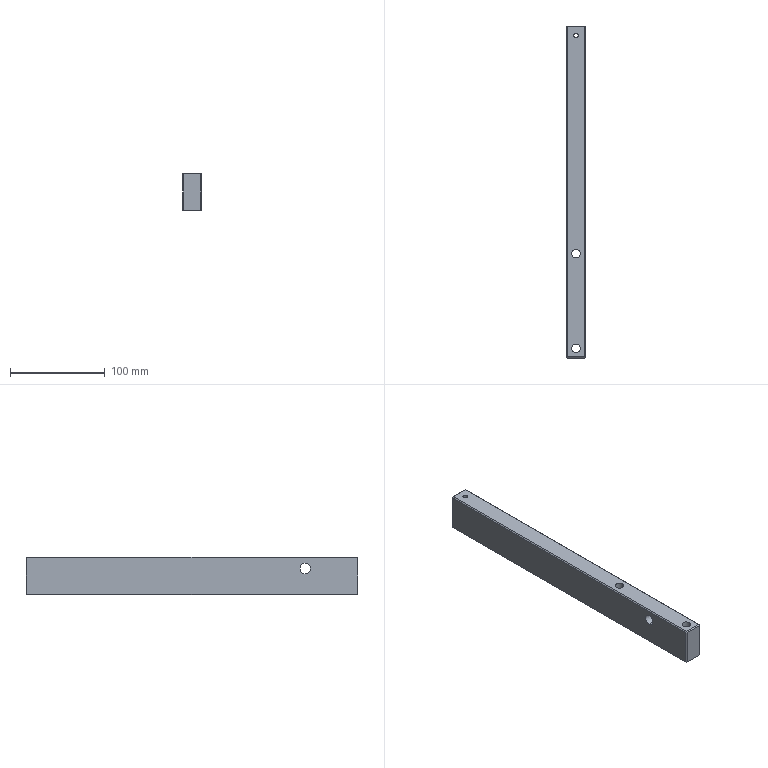Part | SolidWorks | features HoleWzd 3, Chamfer 1, Extrusion 1, ICE 1 | 1 solid | 48 faces | box 20 x 350 x 40 mm | volume 265293 mm3 | plane 30 | cylinder 18 | commonest cylinder face diameters 5 x4 9 x4 15 x4 11 x2 12.8 x2 18 x2
STEP:
#1=CARTESIAN_POINT('',(-1.,55.662,17.));
#2=VERTEX_POINT('',#1);
#3=CARTESIAN_POINT('',(-1.,55.662,-1.));
#4=VERTEX_POINT('',#3);
#5=CARTESIAN_POINT('',(-1.,55.662,8.));
#6=DIRECTION('',(1.,0.,0.));
#7=DIRECTION('',(0.,0.,-1.));
#8=AXIS2_PLACEMENT_3D('',#5,#6,#7);
#9=CIRCLE('',#8,9.);
#10=EDGE_CURVE('',#2,#4,#9,.T.);
#11=ORIENTED_EDGE('',*,*,#10,.F.);
#12=CARTESIAN_POINT('',(10.,55.662,17.));
#13=VERTEX_POINT('',#12);
#14=CARTESIAN_POINT('',(10.,55.662,17.));
#15=DIRECTION('',(1.,0.,0.));
#16=VECTOR('',#15,1000.);
#17=LINE('',#14,#16);
#18=EDGE_CURVE('',#2,#13,#17,.T.);
#19=ORIENTED_EDGE('',*,*,#18,.T.);
#20=CARTESIAN_POINT('',(10.,55.662,-1.));
#21=VERTEX_POINT('',#20);
#22=CARTESIAN_POINT('',(10.,55.662,8.));
#23=DIRECTION('',(1.,0.,0.));
#24=DIRECTION('',(0.,0.,-1.));
#25=AXIS2_PLACEMENT_3D('',#22,#23,#24);
#26=CIRCLE('',#25,9.);
#27=EDGE_CURVE('',#13,#21,#26,.T.);
#28=ORIENTED_EDGE('',*,*,#27,.T.);
#29=CARTESIAN_POINT('',(10.,55.662,-1.));
#30=DIRECTION('',(1.,0.,0.));
#31=VECTOR('',#30,1000.);
#32=LINE('',#29,#31);
#33=EDGE_CURVE('',#4,#21,#32,.T.);
#34=ORIENTED_EDGE('',*,*,#33,.F.);
#35=EDGE_LOOP('',(#11,#19,#28,#34));
#36=FACE_OUTER_BOUND('',#35,.T.);
#37=CARTESIAN_POINT('',(10.,55.662,8.));
#38=DIRECTION('',(1.,0.,0.));
#39=DIRECTION('',(0.,0.,-1.));
#40=AXIS2_PLACEMENT_3D('',#37,#38,#39);
#41=CYLINDRICAL_SURFACE('',#40,9.);
#42=ADVANCED_FACE('',(#36),#41,.F.);
#43=CARTESIAN_POINT('',(-10.,55.662,13.5));
#44=VERTEX_POINT('',#43);
#45=CARTESIAN_POINT('',(-10.,55.662,2.5));
#46=VERTEX_POINT('',#45);
#47=CARTESIAN_POINT('',(-10.,55.662,8.));
#48=DIRECTION('',(1.,0.,0.));
#49=DIRECTION('',(0.,0.,-1.));
#50=AXIS2_PLACEMENT_3D('',#47,#48,#49);
#51=CIRCLE('',#50,5.5);
#52=EDGE_CURVE('',#44,#46,#51,.T.);
#53=ORIENTED_EDGE('',*,*,#52,.F.);
#54=CARTESIAN_POINT('',(-1.,55.662,13.5));
#55=VERTEX_POINT('',#54);
#56=CARTESIAN_POINT('',(10.,55.662,13.5));
#57=DIRECTION('',(1.,0.,0.));
#58=VECTOR('',#57,1000.);
#59=LINE('',#56,#58);
#60=EDGE_CURVE('',#44,#55,#59,.T.);
#61=ORIENTED_EDGE('',*,*,#60,.T.);
#62=CARTESIAN_POINT('',(-1.,55.662,2.5));
#63=VERTEX_POINT('',#62);
#64=CARTESIAN_POINT('',(-1.,55.662,8.));
#65=DIRECTION('',(1.,0.,0.));
#66=DIRECTION('',(0.,0.,-1.));
#67=AXIS2_PLACEMENT_3D('',#64,#65,#66);
#68=CIRCLE('',#67,5.5);
#69=EDGE_CURVE('',#55,#63,#68,.T.);
#70=ORIENTED_EDGE('',*,*,#69,.T.);
#71=CARTESIAN_POINT('',(10.,55.662,2.5));
#72=DIRECTION('',(1.,0.,0.));
#73=VECTOR('',#72,1000.);
#74=LINE('',#71,#73);
#75=EDGE_CURVE('',#46,#63,#74,.T.);
#76=ORIENTED_EDGE('',*,*,#75,.F.);
#77=EDGE_LOOP('',(#53,#61,#70,#76));
#78=FACE_OUTER_BOUND('',#77,.T.);
#79=CARTESIAN_POINT('',(10.,55.662,8.));
#80=DIRECTION('',(1.,0.,0.));
#81=DIRECTION('',(0.,0.,-1.));
#82=AXIS2_PLACEMENT_3D('',#79,#80,#81);
#83=CYLINDRICAL_SURFACE('',#82,5.5);
#84=ADVANCED_FACE('',(#78),#83,.F.);
#85=CARTESIAN_POINT('',(7.5,10.,-11.));
#86=VERTEX_POINT('',#85);
#87=CARTESIAN_POINT('',(-7.5,10.,-11.));
#88=VERTEX_POINT('',#87);
#89=CARTESIAN_POINT('',(0.,10.,-11.));
#90=DIRECTION('',(0.,0.,-1.));
#91=DIRECTION('',(-1.,0.,0.));
#92=AXIS2_PLACEMENT_3D('',#89,#90,#91);
#93=CIRCLE('',#92,7.5);
#94=EDGE_CURVE('',#86,#88,#93,.T.);
#95=ORIENTED_EDGE('',*,*,#94,.F.);
#96=CARTESIAN_POINT('',(7.5,10.,-20.));
#97=VERTEX_POINT('',#96);
#98=CARTESIAN_POINT('',(7.5,10.,-20.));
#99=DIRECTION('',(0.,0.,-1.));
#100=VECTOR('',#99,1000.);
#101=LINE('',#98,#100);
#102=EDGE_CURVE('',#86,#97,#101,.T.);
#103=ORIENTED_EDGE('',*,*,#102,.T.);
#104=CARTESIAN_POINT('',(-7.5,10.,-20.));
#105=VERTEX_POINT('',#104);
#106=CARTESIAN_POINT('',(0.,10.,-20.));
#107=DIRECTION('',(0.,0.,-1.));
#108=DIRECTION('',(-1.,0.,0.));
#109=AXIS2_PLACEMENT_3D('',#106,#107,#108);
#110=CIRCLE('',#109,7.5);
#111=EDGE_CURVE('',#97,#105,#110,.T.);
#112=ORIENTED_EDGE('',*,*,#111,.T.);
#113=CARTESIAN_POINT('',(-7.5,10.,-20.));
#114=DIRECTION('',(0.,0.,-1.));
#115=VECTOR('',#114,1000.);
#116=LINE('',#113,#115);
#117=EDGE_CURVE('',#88,#105,#116,.T.);
#118=ORIENTED_EDGE('',*,*,#117,.F.);
#119=EDGE_LOOP('',(#95,#103,#112,#118));
#120=FACE_OUTER_BOUND('',#119,.T.);
#121=CARTESIAN_POINT('',(0.,10.,-20.));
#122=DIRECTION('',(0.,0.,-1.));
#123=DIRECTION('',(-1.,0.,0.));
#124=AXIS2_PLACEMENT_3D('',#121,#122,#123);
#125=CYLINDRICAL_SURFACE('',#124,7.5);
#126=ADVANCED_FACE('',(#120),#125,.F.);
#127=CARTESIAN_POINT('',(4.5,10.,20.));
#128=VERTEX_POINT('',#127);
#129=CARTESIAN_POINT('',(-4.5,10.,20.));
#130=VERTEX_POINT('',#129);
#131=CARTESIAN_POINT('',(0.,10.,20.));
#132=DIRECTION('',(0.,0.,-1.));
#133=DIRECTION('',(-1.,0.,0.));
#134=AXIS2_PLACEMENT_3D('',#131,#132,#133);
#135=CIRCLE('',#134,4.5);
#136=EDGE_CURVE('',#128,#130,#135,.T.);
#137=ORIENTED_EDGE('',*,*,#136,.F.);
#138=CARTESIAN_POINT('',(4.5,10.,-11.));
#139=VERTEX_POINT('',#138);
#140=CARTESIAN_POINT('',(4.5,10.,-20.));
#141=DIRECTION('',(0.,0.,-1.));
#142=VECTOR('',#141,1000.);
#143=LINE('',#140,#142);
#144=EDGE_CURVE('',#128,#139,#143,.T.);
#145=ORIENTED_EDGE('',*,*,#144,.T.);
#146=CARTESIAN_POINT('',(-4.5,10.,-11.));
#147=VERTEX_POINT('',#146);
#148=CARTESIAN_POINT('',(0.,10.,-11.));
#149=DIRECTION('',(0.,0.,-1.));
#150=DIRECTION('',(-1.,0.,0.));
#151=AXIS2_PLACEMENT_3D('',#148,#149,#150);
#152=CIRCLE('',#151,4.5);
#153=EDGE_CURVE('',#139,#147,#152,.T.);
#154=ORIENTED_EDGE('',*,*,#153,.T.);
#155=CARTESIAN_POINT('',(-4.5,10.,-20.));
#156=DIRECTION('',(0.,0.,-1.));
#157=VECTOR('',#156,1000.);
#158=LINE('',#155,#157);
#159=EDGE_CURVE('',#130,#147,#158,.T.);
#160=ORIENTED_EDGE('',*,*,#159,.F.);
#161=EDGE_LOOP('',(#137,#145,#154,#160));
#162=FACE_OUTER_BOUND('',#161,.T.);
#163=CARTESIAN_POINT('',(0.,10.,-20.));
#164=DIRECTION('',(0.,0.,-1.));
#165=DIRECTION('',(-1.,0.,0.));
#166=AXIS2_PLACEMENT_3D('',#163,#164,#165);
#167=CYLINDRICAL_SURFACE('',#166,4.5);
#168=ADVANCED_FACE('',(#162),#167,.F.);
#169=CARTESIAN_POINT('',(7.5,110.,-11.));
#170=VERTEX_POINT('',#169);
#171=CARTESIAN_POINT('',(-7.5,110.,-11.));
#172=VERTEX_POINT('',#171);
#173=CARTESIAN_POINT('',(0.,110.,-11.));
#174=DIRECTION('',(0.,0.,-1.));
#175=DIRECTION('',(-1.,0.,0.));
#176=AXIS2_PLACEMENT_3D('',#173,#174,#175);
#177=CIRCLE('',#176,7.5);
#178=EDGE_CURVE('',#170,#172,#177,.T.);
#179=ORIENTED_EDGE('',*,*,#178,.F.);
#180=CARTESIAN_POINT('',(7.5,110.,-20.));
#181=VERTEX_POINT('',#180);
#182=CARTESIAN_POINT('',(7.5,110.,-20.));
#183=DIRECTION('',(0.,0.,-1.));
#184=VECTOR('',#183,1000.);
#185=LINE('',#182,#184);
#186=EDGE_CURVE('',#170,#181,#185,.T.);
#187=ORIENTED_EDGE('',*,*,#186,.T.);
#188=CARTESIAN_POINT('',(-7.5,110.,-20.));
#189=VERTEX_POINT('',#188);
#190=CARTESIAN_POINT('',(0.,110.,-20.));
#191=DIRECTION('',(0.,0.,-1.));
#192=DIRECTION('',(-1.,0.,0.));
#193=AXIS2_PLACEMENT_3D('',#190,#191,#192);
#194=CIRCLE('',#193,7.5);
#195=EDGE_CURVE('',#181,#189,#194,.T.);
#196=ORIENTED_EDGE('',*,*,#195,.T.);
#197=CARTESIAN_POINT('',(-7.5,110.,-20.));
#198=DIRECTION('',(0.,0.,-1.));
#199=VECTOR('',#198,1000.);
#200=LINE('',#197,#199);
#201=EDGE_CURVE('',#172,#189,#200,.T.);
#202=ORIENTED_EDGE('',*,*,#201,.F.);
#203=EDGE_LOOP('',(#179,#187,#196,#202));
#204=FACE_OUTER_BOUND('',#203,.T.);
#205=CARTESIAN_POINT('',(0.,110.,-20.));
#206=DIRECTION('',(0.,0.,-1.));
#207=DIRECTION('',(-1.,0.,0.));
#208=AXIS2_PLACEMENT_3D('',#205,#206,#207);
#209=CYLINDRICAL_SURFACE('',#208,7.5);
#210=ADVANCED_FACE('',(#204),#209,.F.);
#211=CARTESIAN_POINT('',(4.5,110.,20.));
#212=VERTEX_POINT('',#211);
#213=CARTESIAN_POINT('',(-4.5,110.,20.));
#214=VERTEX_POINT('',#213);
#215=CARTESIAN_POINT('',(0.,110.,20.));
#216=DIRECTION('',(0.,0.,-1.));
#217=DIRECTION('',(-1.,0.,0.));
#218=AXIS2_PLACEMENT_3D('',#215,#216,#217);
#219=CIRCLE('',#218,4.5);
#220=EDGE_CURVE('',#212,#214,#219,.T.);
#221=ORIENTED_EDGE('',*,*,#220,.F.);
#222=CARTESIAN_POINT('',(4.5,110.,-11.));
#223=VERTEX_POINT('',#222);
#224=CARTESIAN_POINT('',(4.5,110.,-20.));
#225=DIRECTION('',(0.,0.,-1.));
#226=VECTOR('',#225,1000.);
#227=LINE('',#224,#226);
#228=EDGE_CURVE('',#212,#223,#227,.T.);
#229=ORIENTED_EDGE('',*,*,#228,.T.);
#230=CARTESIAN_POINT('',(-4.5,110.,-11.));
#231=VERTEX_POINT('',#230);
#232=CARTESIAN_POINT('',(0.,110.,-11.));
#233=DIRECTION('',(0.,0.,-1.));
#234=DIRECTION('',(-1.,0.,0.));
#235=AXIS2_PLACEMENT_3D('',#232,#233,#234);
#236=CIRCLE('',#235,4.5);
#237=EDGE_CURVE('',#223,#231,#236,.T.);
#238=ORIENTED_EDGE('',*,*,#237,.T.);
#239=CARTESIAN_POINT('',(-4.5,110.,-20.));
#240=DIRECTION('',(0.,0.,-1.));
#241=VECTOR('',#240,1000.);
#242=LINE('',#239,#241);
#243=EDGE_CURVE('',#214,#231,#242,.T.);
#244=ORIENTED_EDGE('',*,*,#243,.F.);
#245=EDGE_LOOP('',(#221,#229,#238,#244));
#246=FACE_OUTER_BOUND('',#245,.T.);
#247=CARTESIAN_POINT('',(0.,110.,-20.));
#248=DIRECTION('',(0.,0.,-1.));
#249=DIRECTION('',(-1.,0.,0.));
#250=AXIS2_PLACEMENT_3D('',#247,#248,#249);
#251=CYLINDRICAL_SURFACE('',#250,4.5);
#252=ADVANCED_FACE('',(#246),#251,.F.);
#253=CARTESIAN_POINT('',(2.5,340.,20.));
#254=VERTEX_POINT('',#253);
#255=CARTESIAN_POINT('',(-2.5,340.,20.));
#256=VERTEX_POINT('',#255);
#257=CARTESIAN_POINT('',(0.,340.,20.));
#258=DIRECTION('',(0.,0.,-1.));
#259=DIRECTION('',(-1.,0.,0.));
#260=AXIS2_PLACEMENT_3D('',#257,#258,#259);
#261=CIRCLE('',#260,2.5);
#262=EDGE_CURVE('',#254,#256,#261,.T.);
#263=ORIENTED_EDGE('',*,*,#262,.F.);
#264=CARTESIAN_POINT('',(2.5,340.,5.372));
#265=VERTEX_POINT('',#264);
#266=CARTESIAN_POINT('',(2.5,340.,-20.));
#267=DIRECTION('',(0.,0.,-1.));
#268=VECTOR('',#267,1000.);
#269=LINE('',#266,#268);
#270=EDGE_CURVE('',#254,#265,#269,.T.);
#271=ORIENTED_EDGE('',*,*,#270,.T.);
#272=CARTESIAN_POINT('',(0.,337.5,5.88));
#273=VERTEX_POINT('',#272);
#274=CARTESIAN_POINT('',(0.,337.5,5.88));
#275=CARTESIAN_POINT('',(0.167,337.5,5.88));
#276=CARTESIAN_POINT('',(0.331,337.517,5.873));
#277=CARTESIAN_POINT('',(0.653,337.581,5.849));
#278=CARTESIAN_POINT('',(0.8127,337.63,5.83));
#279=CARTESIAN_POINT('',(1.115,337.756,5.784));
#280=CARTESIAN_POINT('',(1.258,337.833,5.757));
#281=CARTESIAN_POINT('',(1.529,338.015,5.696));
#282=CARTESIAN_POINT('',(1.655,338.12,5.663));
#283=CARTESIAN_POINT('',(1.997,338.462,5.565));
#284=CARTESIAN_POINT('',(2.183,338.738,5.498));
#285=CARTESIAN_POINT('',(2.37,339.189,5.425));
#286=CARTESIAN_POINT('',(2.419,339.348,5.405));
#287=CARTESIAN_POINT('',(2.484,339.672,5.378));
#288=CARTESIAN_POINT('',(2.5,339.835,5.372));
#289=CARTESIAN_POINT('',(2.5,340.,5.372));
#290=B_SPLINE_CURVE_WITH_KNOTS('',3,(#274,#275,#276,#277,#278,#279,#280,#281,#282,#283,#284,#285,#286,#287,#288,#289),.UNSPECIFIED.,.F.,.F.,(4,2,2,2,2,2,2,4),(0.,0.0004937,0.0009873,0.001481,0.001975,0.002962,0.003456,0.003949),.UNSPECIFIED.);
#291=EDGE_CURVE('',#273,#265,#290,.T.);
#292=ORIENTED_EDGE('',*,*,#291,.F.);
#293=CARTESIAN_POINT('',(-2.5,340.,5.372));
#294=VERTEX_POINT('',#293);
#295=CARTESIAN_POINT('',(-2.5,340.,5.372));
#296=CARTESIAN_POINT('',(-2.5,339.835,5.372));
#297=CARTESIAN_POINT('',(-2.484,339.671,5.378));
#298=CARTESIAN_POINT('',(-2.419,339.346,5.405));
#299=CARTESIAN_POINT('',(-2.37,339.188,5.425));
#300=CARTESIAN_POINT('',(-2.244,338.887,5.474));
#301=CARTESIAN_POINT('',(-2.166,338.741,5.503));
#302=CARTESIAN_POINT('',(-1.985,338.471,5.565));
#303=CARTESIAN_POINT('',(-1.882,338.346,5.598));
#304=CARTESIAN_POINT('',(-1.653,338.117,5.664));
#305=CARTESIAN_POINT('',(-1.525,338.013,5.697));
#306=CARTESIAN_POINT('',(-1.256,337.833,5.757));
#307=CARTESIAN_POINT('',(-1.113,337.755,5.784));
#308=CARTESIAN_POINT('',(-0.6565,337.565,5.854));
#309=CARTESIAN_POINT('',(-0.334,337.5,5.88));
#310=CARTESIAN_POINT('',(0.,337.5,5.88));
#311=B_SPLINE_CURVE_WITH_KNOTS('',3,(#295,#296,#297,#298,#299,#300,#301,#302,#303,#304,#305,#306,#307,#308,#309,#310),.UNSPECIFIED.,.F.,.F.,(4,2,2,2,2,2,2,4),(0.01184,0.01233,0.01283,0.01332,0.01382,0.01431,0.0148,0.01579),.UNSPECIFIED.);
#312=EDGE_CURVE('',#294,#273,#311,.T.);
#313=ORIENTED_EDGE('',*,*,#312,.F.);
#314=CARTESIAN_POINT('',(-2.5,340.,-20.));
#315=DIRECTION('',(0.,0.,-1.));
#316=VECTOR('',#315,1000.);
#317=LINE('',#314,#316);
#318=EDGE_CURVE('',#256,#294,#317,.T.);
#319=ORIENTED_EDGE('',*,*,#318,.F.);
#320=EDGE_LOOP('',(#263,#271,#292,#313,#319));
#321=FACE_OUTER_BOUND('',#320,.T.);
#322=CARTESIAN_POINT('',(0.,340.,-20.));
#323=DIRECTION('',(0.,0.,-1.));
#324=DIRECTION('',(-1.,0.,0.));
#325=AXIS2_PLACEMENT_3D('',#322,#323,#324);
#326=CYLINDRICAL_SURFACE('',#325,2.5);
#327=ADVANCED_FACE('',(#321),#326,.F.);
#328=CARTESIAN_POINT('',(2.5,340.,-6.412));
#329=VERTEX_POINT('',#328);
#330=CARTESIAN_POINT('',(0.,337.5,-6.92));
#331=VERTEX_POINT('',#330);
#332=CARTESIAN_POINT('',(2.5,340.,-6.412));
#333=CARTESIAN_POINT('',(2.5,339.836,-6.412));
#334=CARTESIAN_POINT('',(2.484,339.669,-6.419));
#335=CARTESIAN_POINT('',(2.418,339.345,-6.446));
#336=CARTESIAN_POINT('',(2.37,339.189,-6.465));
#337=CARTESIAN_POINT('',(2.245,338.887,-6.514));
#338=CARTESIAN_POINT('',(2.166,338.741,-6.543));
#339=CARTESIAN_POINT('',(1.986,338.473,-6.605));
#340=CARTESIAN_POINT('',(1.883,338.347,-6.638));
#341=CARTESIAN_POINT('',(1.652,338.117,-6.704));
#342=CARTESIAN_POINT('',(1.527,338.014,-6.737));
#343=CARTESIAN_POINT('',(1.258,337.834,-6.797));
#344=CARTESIAN_POINT('',(1.113,337.755,-6.824));
#345=CARTESIAN_POINT('',(0.8105,337.629,-6.87));
#346=CARTESIAN_POINT('',(0.6544,337.582,-6.889));
#347=CARTESIAN_POINT('',(0.3323,337.517,-6.913));
#348=CARTESIAN_POINT('',(0.1647,337.5,-6.92));
#349=CARTESIAN_POINT('',(0.,337.5,-6.92));
#350=B_SPLINE_CURVE_WITH_KNOTS('',3,(#332,#333,#334,#335,#336,#337,#338,#339,#340,#341,#342,#343,#344,#345,#346,#347,#348,#349),.UNSPECIFIED.,.F.,.F.,(4,2,2,2,2,2,2,2,4),(0.007895,0.008388,0.008882,0.009375,0.009868,0.01036,0.01085,0.01135,0.01184),.UNSPECIFIED.);
#351=EDGE_CURVE('',#329,#331,#350,.T.);
#352=ORIENTED_EDGE('',*,*,#351,.F.);
#353=CARTESIAN_POINT('',(2.5,340.,-20.));
#354=VERTEX_POINT('',#353);
#355=CARTESIAN_POINT('',(2.5,340.,-20.));
#356=DIRECTION('',(0.,0.,-1.));
#357=VECTOR('',#356,1000.);
#358=LINE('',#355,#357);
#359=EDGE_CURVE('',#329,#354,#358,.T.);
#360=ORIENTED_EDGE('',*,*,#359,.T.);
#361=CARTESIAN_POINT('',(-2.5,340.,-20.));
#362=VERTEX_POINT('',#361);
#363=CARTESIAN_POINT('',(0.,340.,-20.));
#364=DIRECTION('',(0.,0.,-1.));
#365=DIRECTION('',(-1.,0.,0.));
#366=AXIS2_PLACEMENT_3D('',#363,#364,#365);
#367=CIRCLE('',#366,2.5);
#368=EDGE_CURVE('',#354,#362,#367,.T.);
#369=ORIENTED_EDGE('',*,*,#368,.T.);
#370=CARTESIAN_POINT('',(-2.5,340.,-6.412));
#371=VERTEX_POINT('',#370);
#372=CARTESIAN_POINT('',(-2.5,340.,-20.));
#373=DIRECTION('',(0.,0.,-1.));
#374=VECTOR('',#373,1000.);
#375=LINE('',#372,#374);
#376=EDGE_CURVE('',#371,#362,#375,.T.);
#377=ORIENTED_EDGE('',*,*,#376,.F.);
#378=CARTESIAN_POINT('',(0.,337.5,-6.92));
#379=CARTESIAN_POINT('',(-0.1649,337.5,-6.92));
#380=CARTESIAN_POINT('',(-0.3287,337.516,-6.914));
#381=CARTESIAN_POINT('',(-0.6543,337.581,-6.889));
#382=CARTESIAN_POINT('',(-0.8123,337.63,-6.87));
#383=CARTESIAN_POINT('',(-1.114,337.756,-6.824));
#384=CARTESIAN_POINT('',(-1.259,337.834,-6.796));
#385=CARTESIAN_POINT('',(-1.53,338.016,-6.736));
#386=CARTESIAN_POINT('',(-1.655,338.119,-6.704));
#387=CARTESIAN_POINT('',(-1.884,338.348,-6.638));
#388=CARTESIAN_POINT('',(-1.988,338.476,-6.604));
#389=CARTESIAN_POINT('',(-2.168,338.745,-6.542));
#390=CARTESIAN_POINT('',(-2.245,338.887,-6.514));
#391=CARTESIAN_POINT('',(-2.435,339.344,-6.44));
#392=CARTESIAN_POINT('',(-2.5,339.666,-6.412));
#393=CARTESIAN_POINT('',(-2.5,340.,-6.412));
#394=B_SPLINE_CURVE_WITH_KNOTS('',3,(#378,#379,#380,#381,#382,#383,#384,#385,#386,#387,#388,#389,#390,#391,#392,#393),.UNSPECIFIED.,.F.,.F.,(4,2,2,2,2,2,2,4),(0.01184,0.01233,0.01283,0.01332,0.01381,0.01431,0.0148,0.01579),.UNSPECIFIED.);
#395=EDGE_CURVE('',#331,#371,#394,.T.);
#396=ORIENTED_EDGE('',*,*,#395,.F.);
#397=EDGE_LOOP('',(#352,#360,#369,#377,#396));
#398=FACE_OUTER_BOUND('',#397,.T.);
#399=CARTESIAN_POINT('',(0.,340.,-20.));
#400=DIRECTION('',(0.,0.,-1.));
#401=DIRECTION('',(-1.,0.,0.));
#402=AXIS2_PLACEMENT_3D('',#399,#400,#401);
#403=CYLINDRICAL_SURFACE('',#402,2.5);
#404=ADVANCED_FACE('',(#398),#403,.F.);
#405=CARTESIAN_POINT('',(0.,330.,-6.92));
#406=VERTEX_POINT('',#405);
#407=CARTESIAN_POINT('',(0.,330.,5.88));
#408=VERTEX_POINT('',#407);
#409=CARTESIAN_POINT('',(0.,330.,-0.52));
#410=DIRECTION('',(0.,1.,0.));
#411=DIRECTION('',(0.,0.,1.));
#412=AXIS2_PLACEMENT_3D('',#409,#410,#411);
#413=CIRCLE('',#412,6.4);
#414=EDGE_CURVE('',#406,#408,#413,.T.);
#415=ORIENTED_EDGE('',*,*,#414,.F.);
#416=CARTESIAN_POINT('',(0.,330.,-6.92));
#417=DIRECTION('',(0.,1.,0.));
#418=VECTOR('',#417,1000.);
#419=LINE('',#416,#418);
#420=EDGE_CURVE('',#406,#331,#419,.T.);
#421=ORIENTED_EDGE('',*,*,#420,.T.);
#422=ORIENTED_EDGE('',*,*,#395,.T.);
#423=CARTESIAN_POINT('',(0.,342.5,-6.92));
#424=VERTEX_POINT('',#423);
#425=CARTESIAN_POINT('',(-2.5,340.,-6.412));
#426=CARTESIAN_POINT('',(-2.5,340.167,-6.412));
#427=CARTESIAN_POINT('',(-2.483,340.331,-6.419));
#428=CARTESIAN_POINT('',(-2.419,340.653,-6.445));
#429=CARTESIAN_POINT('',(-2.37,340.812,-6.465));
#430=CARTESIAN_POINT('',(-2.244,341.114,-6.514));
#431=CARTESIAN_POINT('',(-2.167,341.257,-6.543));
#432=CARTESIAN_POINT('',(-1.986,341.528,-6.605));
#433=CARTESIAN_POINT('',(-1.881,341.654,-6.638));
#434=CARTESIAN_POINT('',(-1.539,341.997,-6.737));
#435=CARTESIAN_POINT('',(-1.263,342.182,-6.802));
#436=CARTESIAN_POINT('',(-0.8118,342.37,-6.87));
#437=CARTESIAN_POINT('',(-0.6523,342.419,-6.889));
#438=CARTESIAN_POINT('',(-0.3286,342.484,-6.914));
#439=CARTESIAN_POINT('',(-0.1651,342.5,-6.92));
#440=CARTESIAN_POINT('',(0.,342.5,-6.92));
#441=B_SPLINE_CURVE_WITH_KNOTS('',3,(#425,#426,#427,#428,#429,#430,#431,#432,#433,#434,#435,#436,#437,#438,#439,#440),.UNSPECIFIED.,.F.,.F.,(4,2,2,2,2,2,2,4),(0.,0.0004936,0.0009872,0.001481,0.001974,0.002962,0.003455,0.003949),.UNSPECIFIED.);
#442=EDGE_CURVE('',#371,#424,#441,.T.);
#443=ORIENTED_EDGE('',*,*,#442,.T.);
#444=CARTESIAN_POINT('',(0.,350.,-6.92));
#445=VERTEX_POINT('',#444);
#446=CARTESIAN_POINT('',(0.,330.,-6.92));
#447=DIRECTION('',(0.,1.,0.));
#448=VECTOR('',#447,1000.);
#449=LINE('',#446,#448);
#450=EDGE_CURVE('',#424,#445,#449,.T.);
#451=ORIENTED_EDGE('',*,*,#450,.T.);
#452=CARTESIAN_POINT('',(0.,350.,5.88));
#453=VERTEX_POINT('',#452);
#454=CARTESIAN_POINT('',(0.,350.,-0.52));
#455=DIRECTION('',(0.,1.,0.));
#456=DIRECTION('',(0.,0.,1.));
#457=AXIS2_PLACEMENT_3D('',#454,#455,#456);
#458=CIRCLE('',#457,6.4);
#459=EDGE_CURVE('',#445,#453,#458,.T.);
#460=ORIENTED_EDGE('',*,*,#459,.T.);
#461=CARTESIAN_POINT('',(0.,342.5,5.88));
#462=VERTEX_POINT('',#461);
#463=CARTESIAN_POINT('',(0.,330.,5.88));
#464=DIRECTION('',(0.,1.,0.));
#465=VECTOR('',#464,1000.);
#466=LINE('',#463,#465);
#467=EDGE_CURVE('',#462,#453,#466,.T.);
#468=ORIENTED_EDGE('',*,*,#467,.F.);
#469=CARTESIAN_POINT('',(0.,342.5,5.88));
#470=CARTESIAN_POINT('',(-0.1644,342.5,5.88));
#471=CARTESIAN_POINT('',(-0.3309,342.484,5.874));
#472=CARTESIAN_POINT('',(-0.6549,342.418,5.848));
#473=CARTESIAN_POINT('',(-0.8113,342.37,5.83));
#474=CARTESIAN_POINT('',(-1.114,342.244,5.784));
#475=CARTESIAN_POINT('',(-1.259,342.166,5.756));
#476=CARTESIAN_POINT('',(-1.528,341.985,5.696));
#477=CARTESIAN_POINT('',(-1.654,341.882,5.664));
#478=CARTESIAN_POINT('',(-1.884,341.651,5.597));
#479=CARTESIAN_POINT('',(-1.987,341.526,5.565));
#480=CARTESIAN_POINT('',(-2.167,341.258,5.503));
#481=CARTESIAN_POINT('',(-2.245,341.112,5.474));
#482=CARTESIAN_POINT('',(-2.371,340.81,5.425));
#483=CARTESIAN_POINT('',(-2.418,340.654,5.406));
#484=CARTESIAN_POINT('',(-2.483,340.332,5.379));
#485=CARTESIAN_POINT('',(-2.5,340.165,5.372));
#486=CARTESIAN_POINT('',(-2.5,340.,5.372));
#487=B_SPLINE_CURVE_WITH_KNOTS('',3,(#469,#470,#471,#472,#473,#474,#475,#476,#477,#478,#479,#480,#481,#482,#483,#484,#485,#486),.UNSPECIFIED.,.F.,.F.,(4,2,2,2,2,2,2,2,4),(0.007896,0.008389,0.008882,0.009375,0.009868,0.01036,0.01085,0.01135,0.01184),.UNSPECIFIED.);
#488=EDGE_CURVE('',#462,#294,#487,.T.);
#489=ORIENTED_EDGE('',*,*,#488,.T.);
#490=ORIENTED_EDGE('',*,*,#312,.T.);
#491=CARTESIAN_POINT('',(0.,330.,5.88));
#492=DIRECTION('',(0.,1.,0.));
#493=VECTOR('',#492,1000.);
#494=LINE('',#491,#493);
#495=EDGE_CURVE('',#408,#273,#494,.T.);
#496=ORIENTED_EDGE('',*,*,#495,.F.);
#497=EDGE_LOOP('',(#415,#421,#422,#443,#451,#460,#468,#489,#490,#496));
#498=FACE_OUTER_BOUND('',#497,.T.);
#499=CARTESIAN_POINT('',(0.,330.,-0.52));
#500=DIRECTION('',(0.,1.,0.));
#501=DIRECTION('',(0.,0.,1.));
#502=AXIS2_PLACEMENT_3D('',#499,#500,#501);
#503=CYLINDRICAL_SURFACE('',#502,6.4);
#504=ADVANCED_FACE('',(#498),#503,.F.);
#505=CARTESIAN_POINT('',(10.,55.662,8.));
#506=DIRECTION('',(1.,0.,0.));
#507=DIRECTION('',(0.,0.,-1.));
#508=AXIS2_PLACEMENT_3D('',#505,#506,#507);
#509=CIRCLE('',#508,9.);
#510=EDGE_CURVE('',#21,#13,#509,.T.);
#511=ORIENTED_EDGE('',*,*,#510,.F.);
#512=ORIENTED_EDGE('',*,*,#27,.F.);
#513=EDGE_LOOP('',(#511,#512));
#514=FACE_BOUND('',#513,.T.);
#515=CARTESIAN_POINT('',(10.,1.,19.));
#516=VERTEX_POINT('',#515);
#517=CARTESIAN_POINT('',(10.,1.,-19.));
#518=VERTEX_POINT('',#517);
#519=CARTESIAN_POINT('',(10.,1.,-20.));
#520=DIRECTION('',(0.,0.,-1.));
#521=VECTOR('',#520,1000.);
#522=LINE('',#519,#521);
#523=EDGE_CURVE('',#516,#518,#522,.T.);
#524=ORIENTED_EDGE('',*,*,#523,.T.);
#525=CARTESIAN_POINT('',(10.,349.,-19.));
#526=VERTEX_POINT('',#525);
#527=CARTESIAN_POINT('',(10.,350.,-19.));
#528=DIRECTION('',(0.,1.,0.));
#529=VECTOR('',#528,1000.);
#530=LINE('',#527,#529);
#531=EDGE_CURVE('',#518,#526,#530,.T.);
#532=ORIENTED_EDGE('',*,*,#531,.T.);
#533=CARTESIAN_POINT('',(10.,349.,19.));
#534=VERTEX_POINT('',#533);
#535=CARTESIAN_POINT('',(10.,349.,20.));
#536=DIRECTION('',(0.,0.,1.));
#537=VECTOR('',#536,1000.);
#538=LINE('',#535,#537);
#539=EDGE_CURVE('',#526,#534,#538,.T.);
#540=ORIENTED_EDGE('',*,*,#539,.T.);
#541=CARTESIAN_POINT('',(10.,350.,19.));
#542=DIRECTION('',(0.,-1.,0.));
#543=VECTOR('',#542,1000.);
#544=LINE('',#541,#543);
#545=EDGE_CURVE('',#534,#516,#544,.T.);
#546=ORIENTED_EDGE('',*,*,#545,.T.);
#547=EDGE_LOOP('',(#524,#532,#540,#546));
#548=FACE_OUTER_BOUND('',#547,.T.);
#549=CARTESIAN_POINT('',(10.,350.,20.));
#550=DIRECTION('',(-1.,0.,0.));
#551=DIRECTION('',(0.,0.,1.));
#552=AXIS2_PLACEMENT_3D('',#549,#550,#551);
#553=PLANE('',#552);
#554=ADVANCED_FACE('',(#514,#548),#553,.F.);
#555=CARTESIAN_POINT('',(0.,10.,-20.));
#556=DIRECTION('',(0.,0.,-1.));
#557=DIRECTION('',(-1.,0.,0.));
#558=AXIS2_PLACEMENT_3D('',#555,#556,#557);
#559=CIRCLE('',#558,7.5);
#560=EDGE_CURVE('',#105,#97,#559,.T.);
#561=ORIENTED_EDGE('',*,*,#560,.F.);
#562=ORIENTED_EDGE('',*,*,#111,.F.);
#563=EDGE_LOOP('',(#561,#562));
#564=FACE_BOUND('',#563,.T.);
#565=CARTESIAN_POINT('',(0.,110.,-20.));
#566=DIRECTION('',(0.,0.,-1.));
#567=DIRECTION('',(-1.,0.,0.));
#568=AXIS2_PLACEMENT_3D('',#565,#566,#567);
#569=CIRCLE('',#568,7.5);
#570=EDGE_CURVE('',#189,#181,#569,.T.);
#571=ORIENTED_EDGE('',*,*,#570,.F.);
#572=ORIENTED_EDGE('',*,*,#195,.F.);
#573=EDGE_LOOP('',(#571,#572));
#574=FACE_BOUND('',#573,.T.);
#575=CARTESIAN_POINT('',(-9.,1.,-20.));
#576=VERTEX_POINT('',#575);
#577=CARTESIAN_POINT('',(-9.,349.,-20.));
#578=VERTEX_POINT('',#577);
#579=CARTESIAN_POINT('',(-9.,350.,-20.));
#580=DIRECTION('',(0.,1.,0.));
#581=VECTOR('',#580,1000.);
#582=LINE('',#579,#581);
#583=EDGE_CURVE('',#576,#578,#582,.T.);
#584=ORIENTED_EDGE('',*,*,#583,.T.);
#585=CARTESIAN_POINT('',(9.,349.,-20.));
#586=VERTEX_POINT('',#585);
#587=CARTESIAN_POINT('',(-10.,349.,-20.));
#588=DIRECTION('',(1.,0.,0.));
#589=VECTOR('',#588,1000.);
#590=LINE('',#587,#589);
#591=EDGE_CURVE('',#578,#586,#590,.T.);
#592=ORIENTED_EDGE('',*,*,#591,.T.);
#593=CARTESIAN_POINT('',(9.,1.,-20.));
#594=VERTEX_POINT('',#593);
#595=CARTESIAN_POINT('',(9.,350.,-20.));
#596=DIRECTION('',(0.,-1.,0.));
#597=VECTOR('',#596,1000.);
#598=LINE('',#595,#597);
#599=EDGE_CURVE('',#586,#594,#598,.T.);
#600=ORIENTED_EDGE('',*,*,#599,.T.);
#601=CARTESIAN_POINT('',(-10.,1.,-20.));
#602=DIRECTION('',(-1.,0.,0.));
#603=VECTOR('',#602,1000.);
#604=LINE('',#601,#603);
#605=EDGE_CURVE('',#594,#576,#604,.T.);
#606=ORIENTED_EDGE('',*,*,#605,.T.);
#607=EDGE_LOOP('',(#584,#592,#600,#606));
#608=FACE_OUTER_BOUND('',#607,.T.);
#609=CARTESIAN_POINT('',(0.,340.,-20.));
#610=DIRECTION('',(0.,0.,-1.));
#611=DIRECTION('',(-1.,0.,0.));
#612=AXIS2_PLACEMENT_3D('',#609,#610,#611);
#613=CIRCLE('',#612,2.5);
#614=EDGE_CURVE('',#362,#354,#613,.T.);
#615=ORIENTED_EDGE('',*,*,#614,.F.);
#616=ORIENTED_EDGE('',*,*,#368,.F.);
#617=EDGE_LOOP('',(#615,#616));
#618=FACE_BOUND('',#617,.T.);
#619=CARTESIAN_POINT('',(-10.,350.,-20.));
#620=DIRECTION('',(0.,0.,1.));
#621=DIRECTION('',(1.,0.,0.));
#622=AXIS2_PLACEMENT_3D('',#619,#620,#621);
#623=PLANE('',#622);
#624=ADVANCED_FACE('',(#564,#574,#608,#618),#623,.F.);
#625=CARTESIAN_POINT('',(-10.,55.662,8.));
#626=DIRECTION('',(1.,0.,0.));
#627=DIRECTION('',(0.,0.,-1.));
#628=AXIS2_PLACEMENT_3D('',#625,#626,#627);
#629=CIRCLE('',#628,5.5);
#630=EDGE_CURVE('',#46,#44,#629,.T.);
#631=ORIENTED_EDGE('',*,*,#630,.T.);
#632=ORIENTED_EDGE('',*,*,#52,.T.);
#633=EDGE_LOOP('',(#631,#632));
#634=FACE_BOUND('',#633,.T.);
#635=CARTESIAN_POINT('',(-10.,1.,19.));
#636=VERTEX_POINT('',#635);
#637=CARTESIAN_POINT('',(-10.,349.,19.));
#638=VERTEX_POINT('',#637);
#639=CARTESIAN_POINT('',(-10.,350.,19.));
#640=DIRECTION('',(0.,1.,0.));
#641=VECTOR('',#640,1000.);
#642=LINE('',#639,#641);
#643=EDGE_CURVE('',#636,#638,#642,.T.);
#644=ORIENTED_EDGE('',*,*,#643,.T.);
#645=CARTESIAN_POINT('',(-10.,349.,-19.));
#646=VERTEX_POINT('',#645);
#647=CARTESIAN_POINT('',(-10.,349.,20.));
#648=DIRECTION('',(0.,0.,-1.));
#649=VECTOR('',#648,1000.);
#650=LINE('',#647,#649);
#651=EDGE_CURVE('',#638,#646,#650,.T.);
#652=ORIENTED_EDGE('',*,*,#651,.T.);
#653=CARTESIAN_POINT('',(-10.,1.,-19.));
#654=VERTEX_POINT('',#653);
#655=CARTESIAN_POINT('',(-10.,350.,-19.));
#656=DIRECTION('',(0.,-1.,0.));
#657=VECTOR('',#656,1000.);
#658=LINE('',#655,#657);
#659=EDGE_CURVE('',#646,#654,#658,.T.);
#660=ORIENTED_EDGE('',*,*,#659,.T.);
#661=CARTESIAN_POINT('',(-10.,1.,20.));
#662=DIRECTION('',(0.,0.,1.));
#663=VECTOR('',#662,1000.);
#664=LINE('',#661,#663);
#665=EDGE_CURVE('',#654,#636,#664,.T.);
#666=ORIENTED_EDGE('',*,*,#665,.T.);
#667=EDGE_LOOP('',(#644,#652,#660,#666));
#668=FACE_OUTER_BOUND('',#667,.T.);
#669=CARTESIAN_POINT('',(-10.,350.,20.));
#670=DIRECTION('',(1.,0.,0.));
#671=DIRECTION('',(0.,0.,-1.));
#672=AXIS2_PLACEMENT_3D('',#669,#670,#671);
#673=PLANE('',#672);
#674=ADVANCED_FACE('',(#634,#668),#673,.F.);
#675=CARTESIAN_POINT('',(0.,10.,20.));
#676=DIRECTION('',(0.,0.,-1.));
#677=DIRECTION('',(-1.,0.,0.));
#678=AXIS2_PLACEMENT_3D('',#675,#676,#677);
#679=CIRCLE('',#678,4.5);
#680=EDGE_CURVE('',#130,#128,#679,.T.);
#681=ORIENTED_EDGE('',*,*,#680,.T.);
#682=ORIENTED_EDGE('',*,*,#136,.T.);
#683=EDGE_LOOP('',(#681,#682));
#684=FACE_BOUND('',#683,.T.);
#685=CARTESIAN_POINT('',(0.,110.,20.));
#686=DIRECTION('',(0.,0.,-1.));
#687=DIRECTION('',(-1.,0.,0.));
#688=AXIS2_PLACEMENT_3D('',#685,#686,#687);
#689=CIRCLE('',#688,4.5);
#690=EDGE_CURVE('',#214,#212,#689,.T.);
#691=ORIENTED_EDGE('',*,*,#690,.T.);
#692=ORIENTED_EDGE('',*,*,#220,.T.);
#693=EDGE_LOOP('',(#691,#692));
#694=FACE_BOUND('',#693,.T.);
#695=CARTESIAN_POINT('',(9.,349.,20.));
#696=VERTEX_POINT('',#695);
#697=CARTESIAN_POINT('',(-9.,349.,20.));
#698=VERTEX_POINT('',#697);
#699=CARTESIAN_POINT('',(-10.,349.,20.));
#700=DIRECTION('',(-1.,0.,0.));
#701=VECTOR('',#700,1000.);
#702=LINE('',#699,#701);
#703=EDGE_CURVE('',#696,#698,#702,.T.);
#704=ORIENTED_EDGE('',*,*,#703,.T.);
#705=CARTESIAN_POINT('',(-9.,1.,20.));
#706=VERTEX_POINT('',#705);
#707=CARTESIAN_POINT('',(-9.,350.,20.));
#708=DIRECTION('',(0.,-1.,0.));
#709=VECTOR('',#708,1000.);
#710=LINE('',#707,#709);
#711=EDGE_CURVE('',#698,#706,#710,.T.);
#712=ORIENTED_EDGE('',*,*,#711,.T.);
#713=CARTESIAN_POINT('',(9.,1.,20.));
#714=VERTEX_POINT('',#713);
#715=CARTESIAN_POINT('',(10.,1.,20.));
#716=DIRECTION('',(1.,0.,0.));
#717=VECTOR('',#716,1000.);
#718=LINE('',#715,#717);
#719=EDGE_CURVE('',#706,#714,#718,.T.);
#720=ORIENTED_EDGE('',*,*,#719,.T.);
#721=CARTESIAN_POINT('',(9.,350.,20.));
#722=DIRECTION('',(0.,1.,0.));
#723=VECTOR('',#722,1000.);
#724=LINE('',#721,#723);
#725=EDGE_CURVE('',#714,#696,#724,.T.);
#726=ORIENTED_EDGE('',*,*,#725,.T.);
#727=EDGE_LOOP('',(#704,#712,#720,#726));
#728=FACE_OUTER_BOUND('',#727,.T.);
#729=CARTESIAN_POINT('',(0.,340.,20.));
#730=DIRECTION('',(0.,0.,-1.));
#731=DIRECTION('',(-1.,0.,0.));
#732=AXIS2_PLACEMENT_3D('',#729,#730,#731);
#733=CIRCLE('',#732,2.5);
#734=EDGE_CURVE('',#256,#254,#733,.T.);
#735=ORIENTED_EDGE('',*,*,#734,.T.);
#736=ORIENTED_EDGE('',*,*,#262,.T.);
#737=EDGE_LOOP('',(#735,#736));
#738=FACE_BOUND('',#737,.T.);
#739=CARTESIAN_POINT('',(-10.,350.,20.));
#740=DIRECTION('',(0.,0.,-1.));
#741=DIRECTION('',(-1.,0.,0.));
#742=AXIS2_PLACEMENT_3D('',#739,#740,#741);
#743=PLANE('',#742);
#744=ADVANCED_FACE('',(#684,#694,#728,#738),#743,.F.);
#745=CARTESIAN_POINT('',(-9.,350.,-19.));
#746=VERTEX_POINT('',#745);
#747=CARTESIAN_POINT('',(-9.,350.,19.));
#748=VERTEX_POINT('',#747);
#749=CARTESIAN_POINT('',(-9.,350.,0.));
#750=DIRECTION('',(0.,0.,1.));
#751=VECTOR('',#750,1000.);
#752=LINE('',#749,#751);
#753=EDGE_CURVE('',#746,#748,#752,.T.);
#754=ORIENTED_EDGE('',*,*,#753,.T.);
#755=CARTESIAN_POINT('',(9.,350.,19.));
#756=VERTEX_POINT('',#755);
#757=CARTESIAN_POINT('',(0.,350.,19.));
#758=DIRECTION('',(1.,0.,0.));
#759=VECTOR('',#758,1000.);
#760=LINE('',#757,#759);
#761=EDGE_CURVE('',#748,#756,#760,.T.);
#762=ORIENTED_EDGE('',*,*,#761,.T.);
#763=CARTESIAN_POINT('',(9.,350.,-19.));
#764=VERTEX_POINT('',#763);
#765=CARTESIAN_POINT('',(9.,350.,0.));
#766=DIRECTION('',(0.,0.,-1.));
#767=VECTOR('',#766,1000.);
#768=LINE('',#765,#767);
#769=EDGE_CURVE('',#756,#764,#768,.T.);
#770=ORIENTED_EDGE('',*,*,#769,.T.);
#771=CARTESIAN_POINT('',(0.,350.,-19.));
#772=DIRECTION('',(-1.,0.,0.));
#773=VECTOR('',#772,1000.);
#774=LINE('',#771,#773);
#775=EDGE_CURVE('',#764,#746,#774,.T.);
#776=ORIENTED_EDGE('',*,*,#775,.T.);
#777=EDGE_LOOP('',(#754,#762,#770,#776));
#778=FACE_OUTER_BOUND('',#777,.T.);
#779=CARTESIAN_POINT('',(0.,350.,-0.52));
#780=DIRECTION('',(0.,1.,0.));
#781=DIRECTION('',(0.,0.,1.));
#782=AXIS2_PLACEMENT_3D('',#779,#780,#781);
#783=CIRCLE('',#782,6.4);
#784=EDGE_CURVE('',#453,#445,#783,.T.);
#785=ORIENTED_EDGE('',*,*,#784,.F.);
#786=ORIENTED_EDGE('',*,*,#459,.F.);
#787=EDGE_LOOP('',(#785,#786));
#788=FACE_BOUND('',#787,.T.);
#789=CARTESIAN_POINT('',(0.,350.,0.));
#790=DIRECTION('',(0.,-1.,0.));
#791=DIRECTION('',(0.,0.,-1.));
#792=AXIS2_PLACEMENT_3D('',#789,#790,#791);
#793=PLANE('',#792);
#794=ADVANCED_FACE('',(#778,#788),#793,.F.);
#795=CARTESIAN_POINT('',(9.,0.,-19.));
#796=VERTEX_POINT('',#795);
#797=CARTESIAN_POINT('',(9.,0.,19.));
#798=VERTEX_POINT('',#797);
#799=CARTESIAN_POINT('',(9.,0.,20.));
#800=DIRECTION('',(0.,0.,1.));
#801=VECTOR('',#800,1000.);
#802=LINE('',#799,#801);
#803=EDGE_CURVE('',#796,#798,#802,.T.);
#804=ORIENTED_EDGE('',*,*,#803,.T.);
#805=CARTESIAN_POINT('',(-9.,0.,19.));
#806=VERTEX_POINT('',#805);
#807=CARTESIAN_POINT('',(-10.,0.,19.));
#808=DIRECTION('',(-1.,0.,0.));
#809=VECTOR('',#808,1000.);
#810=LINE('',#807,#809);
#811=EDGE_CURVE('',#798,#806,#810,.T.);
#812=ORIENTED_EDGE('',*,*,#811,.T.);
#813=CARTESIAN_POINT('',(-9.,0.,-19.));
#814=VERTEX_POINT('',#813);
#815=CARTESIAN_POINT('',(-9.,0.,-20.));
#816=DIRECTION('',(0.,0.,-1.));
#817=VECTOR('',#816,1000.);
#818=LINE('',#815,#817);
#819=EDGE_CURVE('',#806,#814,#818,.T.);
#820=ORIENTED_EDGE('',*,*,#819,.T.);
#821=CARTESIAN_POINT('',(10.,0.,-19.));
#822=DIRECTION('',(1.,0.,0.));
#823=VECTOR('',#822,1000.);
#824=LINE('',#821,#823);
#825=EDGE_CURVE('',#814,#796,#824,.T.);
#826=ORIENTED_EDGE('',*,*,#825,.T.);
#827=EDGE_LOOP('',(#804,#812,#820,#826));
#828=FACE_OUTER_BOUND('',#827,.T.);
#829=CARTESIAN_POINT('',(0.,0.,0.));
#830=DIRECTION('',(0.,-1.,0.));
#831=DIRECTION('',(0.,0.,-1.));
#832=AXIS2_PLACEMENT_3D('',#829,#830,#831);
#833=PLANE('',#832);
#834=ADVANCED_FACE('',(#828),#833,.T.);
#835=ORIENTED_EDGE('',*,*,#420,.F.);
#836=CARTESIAN_POINT('',(0.,330.,-0.52));
#837=DIRECTION('',(0.,1.,0.));
#838=DIRECTION('',(0.,0.,1.));
#839=AXIS2_PLACEMENT_3D('',#836,#837,#838);
#840=CIRCLE('',#839,6.4);
#841=EDGE_CURVE('',#408,#406,#840,.T.);
#842=ORIENTED_EDGE('',*,*,#841,.F.);
#843=ORIENTED_EDGE('',*,*,#495,.T.);
#844=ORIENTED_EDGE('',*,*,#291,.T.);
#845=CARTESIAN_POINT('',(2.5,340.,5.372));
#846=CARTESIAN_POINT('',(2.5,340.165,5.372));
#847=CARTESIAN_POINT('',(2.483,340.332,5.379));
#848=CARTESIAN_POINT('',(2.418,340.654,5.406));
#849=CARTESIAN_POINT('',(2.371,340.811,5.425));
#850=CARTESIAN_POINT('',(2.243,341.116,5.474));
#851=CARTESIAN_POINT('',(2.166,341.259,5.503));
#852=CARTESIAN_POINT('',(1.986,341.528,5.565));
#853=CARTESIAN_POINT('',(1.881,341.655,5.598));
#854=CARTESIAN_POINT('',(1.652,341.883,5.664));
#855=CARTESIAN_POINT('',(1.527,341.986,5.697));
#856=CARTESIAN_POINT('',(1.257,342.167,5.757));
#857=CARTESIAN_POINT('',(1.112,342.245,5.785));
#858=CARTESIAN_POINT('',(0.8111,342.37,5.83));
#859=CARTESIAN_POINT('',(0.6548,342.418,5.849));
#860=CARTESIAN_POINT('',(0.3295,342.484,5.874));
#861=CARTESIAN_POINT('',(0.1644,342.5,5.88));
#862=CARTESIAN_POINT('',(0.,342.5,5.88));
#863=B_SPLINE_CURVE_WITH_KNOTS('',3,(#845,#846,#847,#848,#849,#850,#851,#852,#853,#854,#855,#856,#857,#858,#859,#860,#861,#862),.UNSPECIFIED.,.F.,.F.,(4,2,2,2,2,2,2,2,4),(0.003949,0.004443,0.004936,0.005429,0.005922,0.006416,0.006909,0.007402,0.007896),.UNSPECIFIED.);
#864=EDGE_CURVE('',#265,#462,#863,.T.);
#865=ORIENTED_EDGE('',*,*,#864,.T.);
#866=ORIENTED_EDGE('',*,*,#467,.T.);
#867=ORIENTED_EDGE('',*,*,#784,.T.);
#868=ORIENTED_EDGE('',*,*,#450,.F.);
#869=CARTESIAN_POINT('',(0.,342.5,-6.92));
#870=CARTESIAN_POINT('',(0.165,342.5,-6.92));
#871=CARTESIAN_POINT('',(0.3324,342.483,-6.913));
#872=CARTESIAN_POINT('',(0.6545,342.418,-6.888));
#873=CARTESIAN_POINT('',(0.8113,342.37,-6.87));
#874=CARTESIAN_POINT('',(1.116,342.243,-6.824));
#875=CARTESIAN_POINT('',(1.259,342.166,-6.796));
#876=CARTESIAN_POINT('',(1.528,341.985,-6.736));
#877=CARTESIAN_POINT('',(1.656,341.88,-6.703));
#878=CARTESIAN_POINT('',(1.884,341.651,-6.638));
#879=CARTESIAN_POINT('',(1.987,341.526,-6.605));
#880=CARTESIAN_POINT('',(2.167,341.257,-6.543));
#881=CARTESIAN_POINT('',(2.246,341.111,-6.514));
#882=CARTESIAN_POINT('',(2.37,340.811,-6.465));
#883=CARTESIAN_POINT('',(2.418,340.655,-6.446));
#884=CARTESIAN_POINT('',(2.484,340.33,-6.419));
#885=CARTESIAN_POINT('',(2.5,340.164,-6.412));
#886=CARTESIAN_POINT('',(2.5,340.,-6.412));
#887=B_SPLINE_CURVE_WITH_KNOTS('',3,(#869,#870,#871,#872,#873,#874,#875,#876,#877,#878,#879,#880,#881,#882,#883,#884,#885,#886),.UNSPECIFIED.,.F.,.F.,(4,2,2,2,2,2,2,2,4),(0.003949,0.004442,0.004935,0.005429,0.005922,0.006415,0.006909,0.007402,0.007895),.UNSPECIFIED.);
#888=EDGE_CURVE('',#424,#329,#887,.T.);
#889=ORIENTED_EDGE('',*,*,#888,.T.);
#890=ORIENTED_EDGE('',*,*,#351,.T.);
#891=EDGE_LOOP('',(#835,#842,#843,#844,#865,#866,#867,#868,#889,#890));
#892=FACE_OUTER_BOUND('',#891,.T.);
#893=CARTESIAN_POINT('',(0.,330.,-0.52));
#894=DIRECTION('',(0.,1.,0.));
#895=DIRECTION('',(0.,0.,1.));
#896=AXIS2_PLACEMENT_3D('',#893,#894,#895);
#897=CYLINDRICAL_SURFACE('',#896,6.4);
#898=ADVANCED_FACE('',(#892),#897,.F.);
#899=ORIENTED_EDGE('',*,*,#841,.T.);
#900=ORIENTED_EDGE('',*,*,#414,.T.);
#901=EDGE_LOOP('',(#899,#900));
#902=FACE_OUTER_BOUND('',#901,.T.);
#903=CARTESIAN_POINT('',(0.,330.,-0.52));
#904=DIRECTION('',(0.,1.,0.));
#905=DIRECTION('',(0.,0.,1.));
#906=AXIS2_PLACEMENT_3D('',#903,#904,#905);
#907=PLANE('',#906);
#908=ADVANCED_FACE('',(#902),#907,.T.);
#909=ORIENTED_EDGE('',*,*,#359,.F.);
#910=ORIENTED_EDGE('',*,*,#888,.F.);
#911=ORIENTED_EDGE('',*,*,#442,.F.);
#912=ORIENTED_EDGE('',*,*,#376,.T.);
#913=ORIENTED_EDGE('',*,*,#614,.T.);
#914=EDGE_LOOP('',(#909,#910,#911,#912,#913));
#915=FACE_OUTER_BOUND('',#914,.T.);
#916=CARTESIAN_POINT('',(0.,340.,-20.));
#917=DIRECTION('',(0.,0.,-1.));
#918=DIRECTION('',(-1.,0.,0.));
#919=AXIS2_PLACEMENT_3D('',#916,#917,#918);
#920=CYLINDRICAL_SURFACE('',#919,2.5);
#921=ADVANCED_FACE('',(#915),#920,.F.);
#922=ORIENTED_EDGE('',*,*,#270,.F.);
#923=ORIENTED_EDGE('',*,*,#734,.F.);
#924=ORIENTED_EDGE('',*,*,#318,.T.);
#925=ORIENTED_EDGE('',*,*,#488,.F.);
#926=ORIENTED_EDGE('',*,*,#864,.F.);
#927=EDGE_LOOP('',(#922,#923,#924,#925,#926));
#928=FACE_OUTER_BOUND('',#927,.T.);
#929=CARTESIAN_POINT('',(0.,340.,-20.));
#930=DIRECTION('',(0.,0.,-1.));
#931=DIRECTION('',(-1.,0.,0.));
#932=AXIS2_PLACEMENT_3D('',#929,#930,#931);
#933=CYLINDRICAL_SURFACE('',#932,2.5);
#934=ADVANCED_FACE('',(#928),#933,.F.);
#935=CARTESIAN_POINT('',(-10.,349.,19.));
#936=DIRECTION('',(0.7071,0.,0.7071));
#937=VECTOR('',#936,1000.);
#938=LINE('',#935,#937);
#939=EDGE_CURVE('',#638,#698,#938,.T.);
#940=ORIENTED_EDGE('',*,*,#939,.F.);
#941=ORIENTED_EDGE('',*,*,#643,.F.);
#942=CARTESIAN_POINT('',(-9.,1.,20.));
#943=DIRECTION('',(-0.7071,0.,-0.7071));
#944=VECTOR('',#943,1000.);
#945=LINE('',#942,#944);
#946=EDGE_CURVE('',#706,#636,#945,.T.);
#947=ORIENTED_EDGE('',*,*,#946,.F.);
#948=ORIENTED_EDGE('',*,*,#711,.F.);
#949=EDGE_LOOP('',(#940,#941,#947,#948));
#950=FACE_OUTER_BOUND('',#949,.T.);
#951=CARTESIAN_POINT('',(-9.,350.,20.));
#952=DIRECTION('',(0.7071,0.,-0.7071));
#953=DIRECTION('',(0.,-1.,0.));
#954=AXIS2_PLACEMENT_3D('',#951,#952,#953);
#955=PLANE('',#954);
#956=ADVANCED_FACE('',(#950),#955,.F.);
#957=CARTESIAN_POINT('',(-10.,349.,19.));
#958=DIRECTION('',(0.7071,0.7071,0.));
#959=VECTOR('',#958,1000.);
#960=LINE('',#957,#959);
#961=EDGE_CURVE('',#638,#748,#960,.T.);
#962=ORIENTED_EDGE('',*,*,#961,.F.);
#963=ORIENTED_EDGE('',*,*,#939,.T.);
#964=CARTESIAN_POINT('',(-9.,349.5,19.5));
#965=DIRECTION('',(0.,-0.7071,0.7071));
#966=VECTOR('',#965,1000.);
#967=LINE('',#964,#966);
#968=EDGE_CURVE('',#748,#698,#967,.T.);
#969=ORIENTED_EDGE('',*,*,#968,.F.);
#970=EDGE_LOOP('',(#962,#963,#969));
#971=FACE_OUTER_BOUND('',#970,.T.);
#972=CARTESIAN_POINT('',(-10.,349.,19.));
#973=DIRECTION('',(-0.5774,0.5774,0.5774));
#974=DIRECTION('',(0.7071,0.,0.7071));
#975=AXIS2_PLACEMENT_3D('',#972,#973,#974);
#976=PLANE('',#975);
#977=ADVANCED_FACE('',(#971),#976,.T.);
#978=CARTESIAN_POINT('',(-9.,1.,20.));
#979=DIRECTION('',(0.,-0.7071,-0.7071));
#980=VECTOR('',#979,1000.);
#981=LINE('',#978,#980);
#982=EDGE_CURVE('',#706,#806,#981,.T.);
#983=ORIENTED_EDGE('',*,*,#982,.F.);
#984=ORIENTED_EDGE('',*,*,#946,.T.);
#985=CARTESIAN_POINT('',(-9.5,0.5,19.));
#986=DIRECTION('',(-0.7071,0.7071,0.));
#987=VECTOR('',#986,1000.);
#988=LINE('',#985,#987);
#989=EDGE_CURVE('',#806,#636,#988,.T.);
#990=ORIENTED_EDGE('',*,*,#989,.F.);
#991=EDGE_LOOP('',(#983,#984,#990));
#992=FACE_OUTER_BOUND('',#991,.T.);
#993=CARTESIAN_POINT('',(-9.,1.,20.));
#994=DIRECTION('',(-0.5774,-0.5774,0.5774));
#995=DIRECTION('',(0.7071,-0.7071,0.));
#996=AXIS2_PLACEMENT_3D('',#993,#994,#995);
#997=PLANE('',#996);
#998=ADVANCED_FACE('',(#992),#997,.T.);
#999=ORIENTED_EDGE('',*,*,#968,.T.);
#1000=ORIENTED_EDGE('',*,*,#703,.F.);
#1001=CARTESIAN_POINT('',(9.,350.,19.));
#1002=DIRECTION('',(0.,-0.7071,0.7071));
#1003=VECTOR('',#1002,1000.);
#1004=LINE('',#1001,#1003);
#1005=EDGE_CURVE('',#756,#696,#1004,.T.);
#1006=ORIENTED_EDGE('',*,*,#1005,.F.);
#1007=ORIENTED_EDGE('',*,*,#761,.F.);
#1008=EDGE_LOOP('',(#999,#1000,#1006,#1007));
#1009=FACE_OUTER_BOUND('',#1008,.T.);
#1010=CARTESIAN_POINT('',(0.,350.,19.));
#1011=DIRECTION('',(0.,-0.7071,-0.7071));
#1012=DIRECTION('',(1.,0.,0.));
#1013=AXIS2_PLACEMENT_3D('',#1010,#1011,#1012);
#1014=PLANE('',#1013);
#1015=ADVANCED_FACE('',(#1009),#1014,.F.);
#1016=ORIENTED_EDGE('',*,*,#961,.T.);
#1017=ORIENTED_EDGE('',*,*,#753,.F.);
#1018=CARTESIAN_POINT('',(-9.5,349.5,-19.));
#1019=DIRECTION('',(0.7071,0.7071,0.));
#1020=VECTOR('',#1019,1000.);
#1021=LINE('',#1018,#1020);
#1022=EDGE_CURVE('',#646,#746,#1021,.T.);
#1023=ORIENTED_EDGE('',*,*,#1022,.F.);
#1024=ORIENTED_EDGE('',*,*,#651,.F.);
#1025=EDGE_LOOP('',(#1016,#1017,#1023,#1024));
#1026=FACE_OUTER_BOUND('',#1025,.T.);
#1027=CARTESIAN_POINT('',(-9.,350.,0.));
#1028=DIRECTION('',(0.7071,-0.7071,0.));
#1029=DIRECTION('',(0.,0.,1.));
#1030=AXIS2_PLACEMENT_3D('',#1027,#1028,#1029);
#1031=PLANE('',#1030);
#1032=ADVANCED_FACE('',(#1026),#1031,.F.);
#1033=CARTESIAN_POINT('',(-10.,1.,-19.));
#1034=DIRECTION('',(0.7071,0.,-0.7071));
#1035=VECTOR('',#1034,1000.);
#1036=LINE('',#1033,#1035);
#1037=EDGE_CURVE('',#654,#576,#1036,.T.);
#1038=ORIENTED_EDGE('',*,*,#1037,.F.);
#1039=ORIENTED_EDGE('',*,*,#659,.F.);
#1040=CARTESIAN_POINT('',(-9.,349.,-20.));
#1041=DIRECTION('',(-0.7071,0.,0.7071));
#1042=VECTOR('',#1041,1000.);
#1043=LINE('',#1040,#1042);
#1044=EDGE_CURVE('',#578,#646,#1043,.T.);
#1045=ORIENTED_EDGE('',*,*,#1044,.F.);
#1046=ORIENTED_EDGE('',*,*,#583,.F.);
#1047=EDGE_LOOP('',(#1038,#1039,#1045,#1046));
#1048=FACE_OUTER_BOUND('',#1047,.T.);
#1049=CARTESIAN_POINT('',(-10.,350.,-19.));
#1050=DIRECTION('',(0.7071,0.,0.7071));
#1051=DIRECTION('',(0.,-1.,0.));
#1052=AXIS2_PLACEMENT_3D('',#1049,#1050,#1051);
#1053=PLANE('',#1052);
#1054=ADVANCED_FACE('',(#1048),#1053,.F.);
#1055=ORIENTED_EDGE('',*,*,#989,.T.);
#1056=ORIENTED_EDGE('',*,*,#665,.F.);
#1057=CARTESIAN_POINT('',(-10.,1.,-19.));
#1058=DIRECTION('',(-0.7071,0.7071,0.));
#1059=VECTOR('',#1058,1000.);
#1060=LINE('',#1057,#1059);
#1061=EDGE_CURVE('',#814,#654,#1060,.T.);
#1062=ORIENTED_EDGE('',*,*,#1061,.F.);
#1063=ORIENTED_EDGE('',*,*,#819,.F.);
#1064=EDGE_LOOP('',(#1055,#1056,#1062,#1063));
#1065=FACE_OUTER_BOUND('',#1064,.T.);
#1066=CARTESIAN_POINT('',(-10.,1.,20.));
#1067=DIRECTION('',(-0.7071,-0.7071,0.));
#1068=DIRECTION('',(0.,0.,-1.));
#1069=AXIS2_PLACEMENT_3D('',#1066,#1067,#1068);
#1070=PLANE('',#1069);
#1071=ADVANCED_FACE('',(#1065),#1070,.T.);
#1072=ORIENTED_EDGE('',*,*,#982,.T.);
#1073=ORIENTED_EDGE('',*,*,#811,.F.);
#1074=CARTESIAN_POINT('',(9.,0.5,19.5));
#1075=DIRECTION('',(0.,-0.7071,-0.7071));
#1076=VECTOR('',#1075,1000.);
#1077=LINE('',#1074,#1076);
#1078=EDGE_CURVE('',#714,#798,#1077,.T.);
#1079=ORIENTED_EDGE('',*,*,#1078,.F.);
#1080=ORIENTED_EDGE('',*,*,#719,.F.);
#1081=EDGE_LOOP('',(#1072,#1073,#1079,#1080));
#1082=FACE_OUTER_BOUND('',#1081,.T.);
#1083=CARTESIAN_POINT('',(-10.,1.,20.));
#1084=DIRECTION('',(0.,-0.7071,0.7071));
#1085=DIRECTION('',(-1.,0.,0.));
#1086=AXIS2_PLACEMENT_3D('',#1083,#1084,#1085);
#1087=PLANE('',#1086);
#1088=ADVANCED_FACE('',(#1082),#1087,.T.);
#1089=CARTESIAN_POINT('',(9.5,349.,19.5));
#1090=DIRECTION('',(0.7071,0.,-0.7071));
#1091=VECTOR('',#1090,1000.);
#1092=LINE('',#1089,#1091);
#1093=EDGE_CURVE('',#696,#534,#1092,.T.);
#1094=ORIENTED_EDGE('',*,*,#1093,.F.);
#1095=ORIENTED_EDGE('',*,*,#725,.F.);
#1096=CARTESIAN_POINT('',(10.,1.,19.));
#1097=DIRECTION('',(-0.7071,0.,0.7071));
#1098=VECTOR('',#1097,1000.);
#1099=LINE('',#1096,#1098);
#1100=EDGE_CURVE('',#516,#714,#1099,.T.);
#1101=ORIENTED_EDGE('',*,*,#1100,.F.);
#1102=ORIENTED_EDGE('',*,*,#545,.F.);
#1103=EDGE_LOOP('',(#1094,#1095,#1101,#1102));
#1104=FACE_OUTER_BOUND('',#1103,.T.);
#1105=CARTESIAN_POINT('',(10.,350.,19.));
#1106=DIRECTION('',(-0.7071,0.,-0.7071));
#1107=DIRECTION('',(0.,-1.,0.));
#1108=AXIS2_PLACEMENT_3D('',#1105,#1106,#1107);
#1109=PLANE('',#1108);
#1110=ADVANCED_FACE('',(#1104),#1109,.F.);
#1111=ORIENTED_EDGE('',*,*,#1005,.T.);
#1112=ORIENTED_EDGE('',*,*,#1093,.T.);
#1113=CARTESIAN_POINT('',(9.,350.,19.));
#1114=DIRECTION('',(0.7071,-0.7071,0.));
#1115=VECTOR('',#1114,1000.);
#1116=LINE('',#1113,#1115);
#1117=EDGE_CURVE('',#756,#534,#1116,.T.);
#1118=ORIENTED_EDGE('',*,*,#1117,.F.);
#1119=EDGE_LOOP('',(#1111,#1112,#1118));
#1120=FACE_OUTER_BOUND('',#1119,.T.);
#1121=CARTESIAN_POINT('',(9.,350.,19.));
#1122=DIRECTION('',(0.5774,0.5774,0.5774));
#1123=DIRECTION('',(0.,-0.7071,0.7071));
#1124=AXIS2_PLACEMENT_3D('',#1121,#1122,#1123);
#1125=PLANE('',#1124);
#1126=ADVANCED_FACE('',(#1120),#1125,.T.);
#1127=ORIENTED_EDGE('',*,*,#1044,.T.);
#1128=ORIENTED_EDGE('',*,*,#1022,.T.);
#1129=CARTESIAN_POINT('',(-9.,349.,-20.));
#1130=DIRECTION('',(0.,0.7071,0.7071));
#1131=VECTOR('',#1130,1000.);
#1132=LINE('',#1129,#1131);
#1133=EDGE_CURVE('',#578,#746,#1132,.T.);
#1134=ORIENTED_EDGE('',*,*,#1133,.F.);
#1135=EDGE_LOOP('',(#1127,#1128,#1134));
#1136=FACE_OUTER_BOUND('',#1135,.T.);
#1137=CARTESIAN_POINT('',(-9.,349.,-20.));
#1138=DIRECTION('',(-0.5774,0.5774,-0.5774));
#1139=DIRECTION('',(-0.7071,0.,0.7071));
#1140=AXIS2_PLACEMENT_3D('',#1137,#1138,#1139);
#1141=PLANE('',#1140);
#1142=ADVANCED_FACE('',(#1136),#1141,.T.);
#1143=ORIENTED_EDGE('',*,*,#1061,.T.);
#1144=ORIENTED_EDGE('',*,*,#1037,.T.);
#1145=CARTESIAN_POINT('',(-9.,0.5,-19.5));
#1146=DIRECTION('',(0.,0.7071,-0.7071));
#1147=VECTOR('',#1146,1000.);
#1148=LINE('',#1145,#1147);
#1149=EDGE_CURVE('',#814,#576,#1148,.T.);
#1150=ORIENTED_EDGE('',*,*,#1149,.F.);
#1151=EDGE_LOOP('',(#1143,#1144,#1150));
#1152=FACE_OUTER_BOUND('',#1151,.T.);
#1153=CARTESIAN_POINT('',(-10.,1.,-19.));
#1154=DIRECTION('',(-0.5774,-0.5774,-0.5774));
#1155=DIRECTION('',(0.,0.7071,-0.7071));
#1156=AXIS2_PLACEMENT_3D('',#1153,#1154,#1155);
#1157=PLANE('',#1156);
#1158=ADVANCED_FACE('',(#1152),#1157,.T.);
#1159=ORIENTED_EDGE('',*,*,#1100,.T.);
#1160=ORIENTED_EDGE('',*,*,#1078,.T.);
#1161=CARTESIAN_POINT('',(10.,1.,19.));
#1162=DIRECTION('',(-0.7071,-0.7071,0.));
#1163=VECTOR('',#1162,1000.);
#1164=LINE('',#1161,#1163);
#1165=EDGE_CURVE('',#516,#798,#1164,.T.);
#1166=ORIENTED_EDGE('',*,*,#1165,.F.);
#1167=EDGE_LOOP('',(#1159,#1160,#1166));
#1168=FACE_OUTER_BOUND('',#1167,.T.);
#1169=CARTESIAN_POINT('',(10.,1.,19.));
#1170=DIRECTION('',(0.5774,-0.5774,0.5774));
#1171=DIRECTION('',(0.,-0.7071,-0.7071));
#1172=AXIS2_PLACEMENT_3D('',#1169,#1170,#1171);
#1173=PLANE('',#1172);
#1174=ADVANCED_FACE('',(#1168),#1173,.T.);
#1175=ORIENTED_EDGE('',*,*,#1117,.T.);
#1176=ORIENTED_EDGE('',*,*,#539,.F.);
#1177=CARTESIAN_POINT('',(10.,349.,-19.));
#1178=DIRECTION('',(0.7071,-0.7071,0.));
#1179=VECTOR('',#1178,1000.);
#1180=LINE('',#1177,#1179);
#1181=EDGE_CURVE('',#764,#526,#1180,.T.);
#1182=ORIENTED_EDGE('',*,*,#1181,.F.);
#1183=ORIENTED_EDGE('',*,*,#769,.F.);
#1184=EDGE_LOOP('',(#1175,#1176,#1182,#1183));
#1185=FACE_OUTER_BOUND('',#1184,.T.);
#1186=CARTESIAN_POINT('',(9.,350.,0.));
#1187=DIRECTION('',(-0.7071,-0.7071,0.));
#1188=DIRECTION('',(0.,0.,-1.));
#1189=AXIS2_PLACEMENT_3D('',#1186,#1187,#1188);
#1190=PLANE('',#1189);
#1191=ADVANCED_FACE('',(#1185),#1190,.F.);
#1192=ORIENTED_EDGE('',*,*,#1133,.T.);
#1193=ORIENTED_EDGE('',*,*,#775,.F.);
#1194=CARTESIAN_POINT('',(9.,349.5,-19.5));
#1195=DIRECTION('',(0.,0.7071,0.7071));
#1196=VECTOR('',#1195,1000.);
#1197=LINE('',#1194,#1196);
#1198=EDGE_CURVE('',#586,#764,#1197,.T.);
#1199=ORIENTED_EDGE('',*,*,#1198,.F.);
#1200=ORIENTED_EDGE('',*,*,#591,.F.);
#1201=EDGE_LOOP('',(#1192,#1193,#1199,#1200));
#1202=FACE_OUTER_BOUND('',#1201,.T.);
#1203=CARTESIAN_POINT('',(0.,350.,-19.));
#1204=DIRECTION('',(0.,-0.7071,0.7071));
#1205=DIRECTION('',(-1.,0.,0.));
#1206=AXIS2_PLACEMENT_3D('',#1203,#1204,#1205);
#1207=PLANE('',#1206);
#1208=ADVANCED_FACE('',(#1202),#1207,.F.);
#1209=ORIENTED_EDGE('',*,*,#1149,.T.);
#1210=ORIENTED_EDGE('',*,*,#605,.F.);
#1211=CARTESIAN_POINT('',(9.,1.,-20.));
#1212=DIRECTION('',(0.,0.7071,-0.7071));
#1213=VECTOR('',#1212,1000.);
#1214=LINE('',#1211,#1213);
#1215=EDGE_CURVE('',#796,#594,#1214,.T.);
#1216=ORIENTED_EDGE('',*,*,#1215,.F.);
#1217=ORIENTED_EDGE('',*,*,#825,.F.);
#1218=EDGE_LOOP('',(#1209,#1210,#1216,#1217));
#1219=FACE_OUTER_BOUND('',#1218,.T.);
#1220=CARTESIAN_POINT('',(-10.,1.,-20.));
#1221=DIRECTION('',(0.,-0.7071,-0.7071));
#1222=DIRECTION('',(1.,0.,0.));
#1223=AXIS2_PLACEMENT_3D('',#1220,#1221,#1222);
#1224=PLANE('',#1223);
#1225=ADVANCED_FACE('',(#1219),#1224,.T.);
#1226=ORIENTED_EDGE('',*,*,#1165,.T.);
#1227=ORIENTED_EDGE('',*,*,#803,.F.);
#1228=CARTESIAN_POINT('',(9.5,0.5,-19.));
#1229=DIRECTION('',(-0.7071,-0.7071,0.));
#1230=VECTOR('',#1229,1000.);
#1231=LINE('',#1228,#1230);
#1232=EDGE_CURVE('',#518,#796,#1231,.T.);
#1233=ORIENTED_EDGE('',*,*,#1232,.F.);
#1234=ORIENTED_EDGE('',*,*,#523,.F.);
#1235=EDGE_LOOP('',(#1226,#1227,#1233,#1234));
#1236=FACE_OUTER_BOUND('',#1235,.T.);
#1237=CARTESIAN_POINT('',(10.,1.,20.));
#1238=DIRECTION('',(0.7071,-0.7071,0.));
#1239=DIRECTION('',(0.,0.,1.));
#1240=AXIS2_PLACEMENT_3D('',#1237,#1238,#1239);
#1241=PLANE('',#1240);
#1242=ADVANCED_FACE('',(#1236),#1241,.T.);
#1243=ORIENTED_EDGE('',*,*,#1198,.T.);
#1244=ORIENTED_EDGE('',*,*,#1181,.T.);
#1245=CARTESIAN_POINT('',(10.,349.,-19.));
#1246=DIRECTION('',(0.7071,0.,0.7071));
#1247=VECTOR('',#1246,1000.);
#1248=LINE('',#1245,#1247);
#1249=EDGE_CURVE('',#586,#526,#1248,.T.);
#1250=ORIENTED_EDGE('',*,*,#1249,.F.);
#1251=EDGE_LOOP('',(#1243,#1244,#1250));
#1252=FACE_OUTER_BOUND('',#1251,.T.);
#1253=CARTESIAN_POINT('',(10.,349.,-19.));
#1254=DIRECTION('',(0.5774,0.5774,-0.5774));
#1255=DIRECTION('',(0.,0.7071,0.7071));
#1256=AXIS2_PLACEMENT_3D('',#1253,#1254,#1255);
#1257=PLANE('',#1256);
#1258=ADVANCED_FACE('',(#1252),#1257,.T.);
#1259=ORIENTED_EDGE('',*,*,#1232,.T.);
#1260=ORIENTED_EDGE('',*,*,#1215,.T.);
#1261=CARTESIAN_POINT('',(9.,1.,-20.));
#1262=DIRECTION('',(-0.7071,0.,-0.7071));
#1263=VECTOR('',#1262,1000.);
#1264=LINE('',#1261,#1263);
#1265=EDGE_CURVE('',#518,#594,#1264,.T.);
#1266=ORIENTED_EDGE('',*,*,#1265,.F.);
#1267=EDGE_LOOP('',(#1259,#1260,#1266));
#1268=FACE_OUTER_BOUND('',#1267,.T.);
#1269=CARTESIAN_POINT('',(9.,1.,-20.));
#1270=DIRECTION('',(0.5774,-0.5774,-0.5774));
#1271=DIRECTION('',(0.,0.7071,-0.7071));
#1272=AXIS2_PLACEMENT_3D('',#1269,#1270,#1271);
#1273=PLANE('',#1272);
#1274=ADVANCED_FACE('',(#1268),#1273,.T.);
#1275=ORIENTED_EDGE('',*,*,#1249,.T.);
#1276=ORIENTED_EDGE('',*,*,#531,.F.);
#1277=ORIENTED_EDGE('',*,*,#1265,.T.);
#1278=ORIENTED_EDGE('',*,*,#599,.F.);
#1279=EDGE_LOOP('',(#1275,#1276,#1277,#1278));
#1280=FACE_OUTER_BOUND('',#1279,.T.);
#1281=CARTESIAN_POINT('',(9.,350.,-20.));
#1282=DIRECTION('',(-0.7071,0.,0.7071));
#1283=DIRECTION('',(0.,-1.,0.));
#1284=AXIS2_PLACEMENT_3D('',#1281,#1282,#1283);
#1285=PLANE('',#1284);
#1286=ADVANCED_FACE('',(#1280),#1285,.F.);
#1287=ORIENTED_EDGE('',*,*,#228,.F.);
#1288=ORIENTED_EDGE('',*,*,#690,.F.);
#1289=ORIENTED_EDGE('',*,*,#243,.T.);
#1290=CARTESIAN_POINT('',(0.,110.,-11.));
#1291=DIRECTION('',(0.,0.,-1.));
#1292=DIRECTION('',(-1.,0.,0.));
#1293=AXIS2_PLACEMENT_3D('',#1290,#1291,#1292);
#1294=CIRCLE('',#1293,4.5);
#1295=EDGE_CURVE('',#231,#223,#1294,.T.);
#1296=ORIENTED_EDGE('',*,*,#1295,.T.);
#1297=EDGE_LOOP('',(#1287,#1288,#1289,#1296));
#1298=FACE_OUTER_BOUND('',#1297,.T.);
#1299=CARTESIAN_POINT('',(0.,110.,-20.));
#1300=DIRECTION('',(0.,0.,-1.));
#1301=DIRECTION('',(-1.,0.,0.));
#1302=AXIS2_PLACEMENT_3D('',#1299,#1300,#1301);
#1303=CYLINDRICAL_SURFACE('',#1302,4.5);
#1304=ADVANCED_FACE('',(#1298),#1303,.F.);
#1305=ORIENTED_EDGE('',*,*,#1295,.F.);
#1306=ORIENTED_EDGE('',*,*,#237,.F.);
#1307=EDGE_LOOP('',(#1305,#1306));
#1308=FACE_BOUND('',#1307,.T.);
#1309=CARTESIAN_POINT('',(0.,110.,-11.));
#1310=DIRECTION('',(0.,0.,-1.));
#1311=DIRECTION('',(-1.,0.,0.));
#1312=AXIS2_PLACEMENT_3D('',#1309,#1310,#1311);
#1313=CIRCLE('',#1312,7.5);
#1314=EDGE_CURVE('',#172,#170,#1313,.T.);
#1315=ORIENTED_EDGE('',*,*,#1314,.T.);
#1316=ORIENTED_EDGE('',*,*,#178,.T.);
#1317=EDGE_LOOP('',(#1315,#1316));
#1318=FACE_OUTER_BOUND('',#1317,.T.);
#1319=CARTESIAN_POINT('',(4.5,110.,-11.));
#1320=DIRECTION('',(0.,0.,1.));
#1321=DIRECTION('',(1.,0.,0.));
#1322=AXIS2_PLACEMENT_3D('',#1319,#1320,#1321);
#1323=PLANE('',#1322);
#1324=ADVANCED_FACE('',(#1308,#1318),#1323,.F.);
#1325=ORIENTED_EDGE('',*,*,#186,.F.);
#1326=ORIENTED_EDGE('',*,*,#1314,.F.);
#1327=ORIENTED_EDGE('',*,*,#201,.T.);
#1328=ORIENTED_EDGE('',*,*,#570,.T.);
#1329=EDGE_LOOP('',(#1325,#1326,#1327,#1328));
#1330=FACE_OUTER_BOUND('',#1329,.T.);
#1331=CARTESIAN_POINT('',(0.,110.,-20.));
#1332=DIRECTION('',(0.,0.,-1.));
#1333=DIRECTION('',(-1.,0.,0.));
#1334=AXIS2_PLACEMENT_3D('',#1331,#1332,#1333);
#1335=CYLINDRICAL_SURFACE('',#1334,7.5);
#1336=ADVANCED_FACE('',(#1330),#1335,.F.);
#1337=ORIENTED_EDGE('',*,*,#144,.F.);
#1338=ORIENTED_EDGE('',*,*,#680,.F.);
#1339=ORIENTED_EDGE('',*,*,#159,.T.);
#1340=CARTESIAN_POINT('',(0.,10.,-11.));
#1341=DIRECTION('',(0.,0.,-1.));
#1342=DIRECTION('',(-1.,0.,0.));
#1343=AXIS2_PLACEMENT_3D('',#1340,#1341,#1342);
#1344=CIRCLE('',#1343,4.5);
#1345=EDGE_CURVE('',#147,#139,#1344,.T.);
#1346=ORIENTED_EDGE('',*,*,#1345,.T.);
#1347=EDGE_LOOP('',(#1337,#1338,#1339,#1346));
#1348=FACE_OUTER_BOUND('',#1347,.T.);
#1349=CARTESIAN_POINT('',(0.,10.,-20.));
#1350=DIRECTION('',(0.,0.,-1.));
#1351=DIRECTION('',(-1.,0.,0.));
#1352=AXIS2_PLACEMENT_3D('',#1349,#1350,#1351);
#1353=CYLINDRICAL_SURFACE('',#1352,4.5);
#1354=ADVANCED_FACE('',(#1348),#1353,.F.);
#1355=ORIENTED_EDGE('',*,*,#1345,.F.);
#1356=ORIENTED_EDGE('',*,*,#153,.F.);
#1357=EDGE_LOOP('',(#1355,#1356));
#1358=FACE_BOUND('',#1357,.T.);
#1359=CARTESIAN_POINT('',(0.,10.,-11.));
#1360=DIRECTION('',(0.,0.,-1.));
#1361=DIRECTION('',(-1.,0.,0.));
#1362=AXIS2_PLACEMENT_3D('',#1359,#1360,#1361);
#1363=CIRCLE('',#1362,7.5);
#1364=EDGE_CURVE('',#88,#86,#1363,.T.);
#1365=ORIENTED_EDGE('',*,*,#1364,.T.);
#1366=ORIENTED_EDGE('',*,*,#94,.T.);
#1367=EDGE_LOOP('',(#1365,#1366));
#1368=FACE_OUTER_BOUND('',#1367,.T.);
#1369=CARTESIAN_POINT('',(4.5,10.,-11.));
#1370=DIRECTION('',(0.,0.,1.));
#1371=DIRECTION('',(1.,0.,0.));
#1372=AXIS2_PLACEMENT_3D('',#1369,#1370,#1371);
#1373=PLANE('',#1372);
#1374=ADVANCED_FACE('',(#1358,#1368),#1373,.F.);
#1375=ORIENTED_EDGE('',*,*,#102,.F.);
#1376=ORIENTED_EDGE('',*,*,#1364,.F.);
#1377=ORIENTED_EDGE('',*,*,#117,.T.);
#1378=ORIENTED_EDGE('',*,*,#560,.T.);
#1379=EDGE_LOOP('',(#1375,#1376,#1377,#1378));
#1380=FACE_OUTER_BOUND('',#1379,.T.);
#1381=CARTESIAN_POINT('',(0.,10.,-20.));
#1382=DIRECTION('',(0.,0.,-1.));
#1383=DIRECTION('',(-1.,0.,0.));
#1384=AXIS2_PLACEMENT_3D('',#1381,#1382,#1383);
#1385=CYLINDRICAL_SURFACE('',#1384,7.5);
#1386=ADVANCED_FACE('',(#1380),#1385,.F.);
#1387=ORIENTED_EDGE('',*,*,#60,.F.);
#1388=ORIENTED_EDGE('',*,*,#630,.F.);
#1389=ORIENTED_EDGE('',*,*,#75,.T.);
#1390=CARTESIAN_POINT('',(-1.,55.662,8.));
#1391=DIRECTION('',(1.,0.,0.));
#1392=DIRECTION('',(0.,0.,-1.));
#1393=AXIS2_PLACEMENT_3D('',#1390,#1391,#1392);
#1394=CIRCLE('',#1393,5.5);
#1395=EDGE_CURVE('',#63,#55,#1394,.T.);
#1396=ORIENTED_EDGE('',*,*,#1395,.T.);
#1397=EDGE_LOOP('',(#1387,#1388,#1389,#1396));
#1398=FACE_OUTER_BOUND('',#1397,.T.);
#1399=CARTESIAN_POINT('',(10.,55.662,8.));
#1400=DIRECTION('',(1.,0.,0.));
#1401=DIRECTION('',(0.,0.,-1.));
#1402=AXIS2_PLACEMENT_3D('',#1399,#1400,#1401);
#1403=CYLINDRICAL_SURFACE('',#1402,5.5);
#1404=ADVANCED_FACE('',(#1398),#1403,.F.);
#1405=ORIENTED_EDGE('',*,*,#1395,.F.);
#1406=ORIENTED_EDGE('',*,*,#69,.F.);
#1407=EDGE_LOOP('',(#1405,#1406));
#1408=FACE_BOUND('',#1407,.T.);
#1409=CARTESIAN_POINT('',(-1.,55.662,8.));
#1410=DIRECTION('',(1.,0.,0.));
#1411=DIRECTION('',(0.,0.,-1.));
#1412=AXIS2_PLACEMENT_3D('',#1409,#1410,#1411);
#1413=CIRCLE('',#1412,9.);
#1414=EDGE_CURVE('',#4,#2,#1413,.T.);
#1415=ORIENTED_EDGE('',*,*,#1414,.T.);
#1416=ORIENTED_EDGE('',*,*,#10,.T.);
#1417=EDGE_LOOP('',(#1415,#1416));
#1418=FACE_OUTER_BOUND('',#1417,.T.);
#1419=CARTESIAN_POINT('',(-1.,61.162,8.));
#1420=DIRECTION('',(-1.,0.,0.));
#1421=DIRECTION('',(0.,0.,1.));
#1422=AXIS2_PLACEMENT_3D('',#1419,#1420,#1421);
#1423=PLANE('',#1422);
#1424=ADVANCED_FACE('',(#1408,#1418),#1423,.F.);
#1425=ORIENTED_EDGE('',*,*,#18,.F.);
#1426=ORIENTED_EDGE('',*,*,#1414,.F.);
#1427=ORIENTED_EDGE('',*,*,#33,.T.);
#1428=ORIENTED_EDGE('',*,*,#510,.T.);
#1429=EDGE_LOOP('',(#1425,#1426,#1427,#1428));
#1430=FACE_OUTER_BOUND('',#1429,.T.);
#1431=CARTESIAN_POINT('',(10.,55.662,8.));
#1432=DIRECTION('',(1.,0.,0.));
#1433=DIRECTION('',(0.,0.,-1.));
#1434=AXIS2_PLACEMENT_3D('',#1431,#1432,#1433);
#1435=CYLINDRICAL_SURFACE('',#1434,9.);
#1436=ADVANCED_FACE('',(#1430),#1435,.F.);
#1437=CLOSED_SHELL('',(#42,#84,#126,#168,#210,#252,#327,#404,#504,#554,#624,#674,#744,#794,#834,#898,#908,#921,#934,#956,#977,#998,#1015,#1032,#1054,#1071,#1088,#1110,#1126,#1142,#1158,#1174,#1191,#1208,#1225,#1242,#1258,#1274,#1286,#1304,#1324,#1336,#1354,#1374,#1386,#1404,#1424,#1436));
#1438=MANIFOLD_SOLID_BREP('',#1437);
#1439=CARTESIAN_POINT('',(0.,0.,0.));
#1440=DIRECTION('',(0.,0.,1.));
#1441=DIRECTION('',(1.,0.,0.));
#1442=AXIS2_PLACEMENT_3D('',#1439,#1440,#1441);
#1443=(LENGTH_UNIT()NAMED_UNIT(*)SI_UNIT(.MILLI.,.METRE.));
#1444=UNCERTAINTY_MEASURE_WITH_UNIT(LENGTH_MEASURE(0.00001),#1443,'','');
#1445=(NAMED_UNIT(*)PLANE_ANGLE_UNIT()SI_UNIT($,.RADIAN.));
#1446=(NAMED_UNIT(*)SI_UNIT($,.STERADIAN.)SOLID_ANGLE_UNIT());
#1447=(GEOMETRIC_REPRESENTATION_CONTEXT(3)GLOBAL_UNCERTAINTY_ASSIGNED_CONTEXT((#1444))GLOBAL_UNIT_ASSIGNED_CONTEXT((#1443,#1445,#1446))REPRESENTATION_CONTEXT('',''));
#1448=ADVANCED_BREP_SHAPE_REPRESENTATION('',(#1438,#1442),#1447);